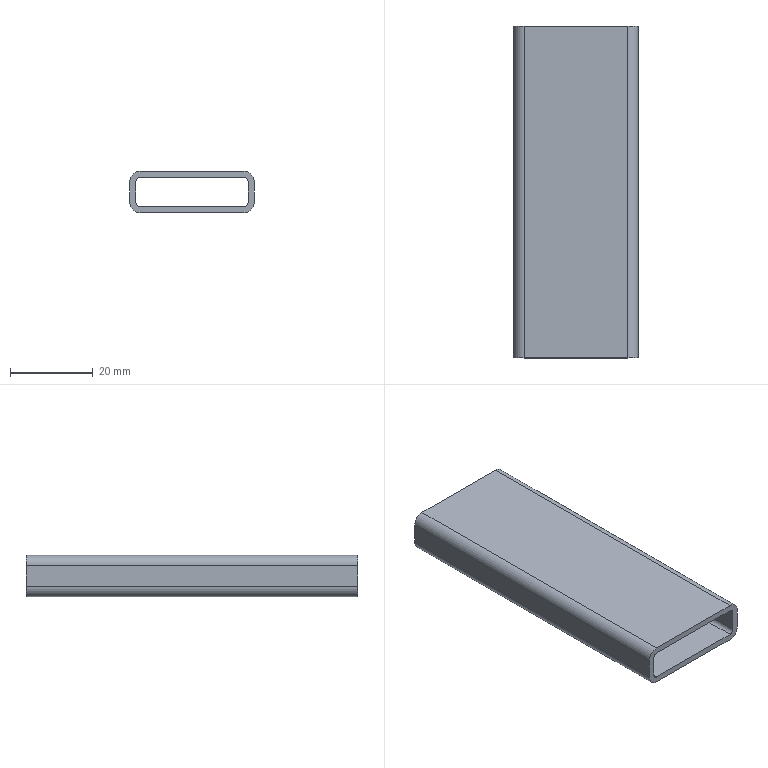Part | STEP file | 7100109 | 1 solid | 18 faces | box 30 x 80 x 10 mm | volume 8519 mm3 | plane 10 | cylinder 8 | commonest cylinder face diameters 2 x4 5 x4
STEP:
#1=CARTESIAN_POINT('',(0.,0.,0.));
#2=DIRECTION('',(0.,0.,1.));
#3=DIRECTION('',(1.,0.,0.));
#4=AXIS2_PLACEMENT_3D('',#1,#2,#3);
#5=CARTESIAN_POINT('',(6.674,80.,-4.725));
#6=VERTEX_POINT('',#5);
#7=CARTESIAN_POINT('',(9.174,80.,-2.225));
#8=VERTEX_POINT('',#7);
#9=CARTESIAN_POINT('',(9.174,80.,-4.725));
#10=DIRECTION('',(0.,1.,0.));
#11=DIRECTION('',(0.,0.,1.));
#12=AXIS2_PLACEMENT_3D('',#9,#10,#11);
#13=CIRCLE('',#12,2.5);
#14=CARTESIAN_POINT('',(9.174,80.,-4.725));
#15=DIRECTION('',(0.,1.,0.));
#16=DIRECTION('',(0.,0.,1.));
#17=AXIS2_PLACEMENT_3D('',#14,#15,#16);
#18=PLANE('',#17);
#19=CARTESIAN_POINT('',(0.,0.));
#20=DIRECTION('',(1.,0.));
#21=AXIS2_PLACEMENT_2D('',#19,#20);
#22=CIRCLE('',#21,2.5);
#23=(GEOMETRIC_REPRESENTATION_CONTEXT(2)PARAMETRIC_REPRESENTATION_CONTEXT()REPRESENTATION_CONTEXT('',''));
#24=DEFINITIONAL_REPRESENTATION('',(#22),#23);
#25=PCURVE('',#18,#24);
#26=CARTESIAN_POINT('',(9.174,80.,-4.725));
#27=DIRECTION('',(0.,-1.,0.));
#28=DIRECTION('',(0.,0.,-1.));
#29=AXIS2_PLACEMENT_3D('',#26,#27,#28);
#30=CYLINDRICAL_SURFACE('',#29,2.5);
#31=CARTESIAN_POINT('',(9.425,0.));
#32=DIRECTION('',(-1.,0.));
#33=VECTOR('',#32,1.);
#34=LINE('',#31,#33);
#35=(GEOMETRIC_REPRESENTATION_CONTEXT(2)PARAMETRIC_REPRESENTATION_CONTEXT()REPRESENTATION_CONTEXT('',''));
#36=DEFINITIONAL_REPRESENTATION('',(#34),#35);
#37=PCURVE('',#30,#36);
#38=SURFACE_CURVE('',#13,(#25,#37),.PCURVE_S1.);
#39=EDGE_CURVE('',#6,#8,#38,.T.);
#40=ORIENTED_EDGE('',*,*,#39,.T.);
#41=CARTESIAN_POINT('',(34.174,80.,-2.225));
#42=VERTEX_POINT('',#41);
#43=CARTESIAN_POINT('',(9.174,80.,-2.225));
#44=DIRECTION('',(1.,0.,0.));
#45=VECTOR('',#44,1.);
#46=LINE('',#43,#45);
#47=CARTESIAN_POINT('',(2.5,0.));
#48=DIRECTION('',(0.,1.));
#49=VECTOR('',#48,1.);
#50=LINE('',#47,#49);
#51=(GEOMETRIC_REPRESENTATION_CONTEXT(2)PARAMETRIC_REPRESENTATION_CONTEXT()REPRESENTATION_CONTEXT('',''));
#52=DEFINITIONAL_REPRESENTATION('',(#50),#51);
#53=PCURVE('',#18,#52);
#54=CARTESIAN_POINT('',(9.174,80.,-2.225));
#55=DIRECTION('',(0.,0.,-1.));
#56=DIRECTION('',(-1.,0.,0.));
#57=AXIS2_PLACEMENT_3D('',#54,#55,#56);
#58=PLANE('',#57);
#59=CARTESIAN_POINT('',(0.,0.));
#60=DIRECTION('',(-1.,0.));
#61=VECTOR('',#60,1.);
#62=LINE('',#59,#61);
#63=(GEOMETRIC_REPRESENTATION_CONTEXT(2)PARAMETRIC_REPRESENTATION_CONTEXT()REPRESENTATION_CONTEXT('',''));
#64=DEFINITIONAL_REPRESENTATION('',(#62),#63);
#65=PCURVE('',#58,#64);
#66=SURFACE_CURVE('',#46,(#53,#65),.PCURVE_S1.);
#67=EDGE_CURVE('',#8,#42,#66,.T.);
#68=ORIENTED_EDGE('',*,*,#67,.T.);
#69=CARTESIAN_POINT('',(36.674,80.,-4.725));
#70=VERTEX_POINT('',#69);
#71=CARTESIAN_POINT('',(34.174,80.,-4.725));
#72=DIRECTION('',(0.,1.,0.));
#73=DIRECTION('',(0.,0.,1.));
#74=AXIS2_PLACEMENT_3D('',#71,#72,#73);
#75=CIRCLE('',#74,2.5);
#76=CARTESIAN_POINT('',(0.,25.));
#77=DIRECTION('',(1.,0.));
#78=AXIS2_PLACEMENT_2D('',#76,#77);
#79=CIRCLE('',#78,2.5);
#80=(GEOMETRIC_REPRESENTATION_CONTEXT(2)PARAMETRIC_REPRESENTATION_CONTEXT()REPRESENTATION_CONTEXT('',''));
#81=DEFINITIONAL_REPRESENTATION('',(#79),#80);
#82=PCURVE('',#18,#81);
#83=CARTESIAN_POINT('',(34.174,80.,-4.725));
#84=DIRECTION('',(0.,-1.,0.));
#85=DIRECTION('',(0.,0.,-1.));
#86=AXIS2_PLACEMENT_3D('',#83,#84,#85);
#87=CYLINDRICAL_SURFACE('',#86,2.5);
#88=CARTESIAN_POINT('',(3.142,0.));
#89=DIRECTION('',(-1.,0.));
#90=VECTOR('',#89,1.);
#91=LINE('',#88,#90);
#92=(GEOMETRIC_REPRESENTATION_CONTEXT(2)PARAMETRIC_REPRESENTATION_CONTEXT()REPRESENTATION_CONTEXT('',''));
#93=DEFINITIONAL_REPRESENTATION('',(#91),#92);
#94=PCURVE('',#87,#93);
#95=SURFACE_CURVE('',#75,(#82,#94),.PCURVE_S1.);
#96=EDGE_CURVE('',#42,#70,#95,.T.);
#97=ORIENTED_EDGE('',*,*,#96,.T.);
#98=CARTESIAN_POINT('',(36.674,80.,-9.725));
#99=VERTEX_POINT('',#98);
#100=CARTESIAN_POINT('',(36.674,80.,-9.725));
#101=DIRECTION('',(0.,0.,-1.));
#102=VECTOR('',#101,1.);
#103=LINE('',#100,#102);
#104=CARTESIAN_POINT('',(-5.,27.5));
#105=DIRECTION('',(-1.,0.));
#106=VECTOR('',#105,1.);
#107=LINE('',#104,#106);
#108=(GEOMETRIC_REPRESENTATION_CONTEXT(2)PARAMETRIC_REPRESENTATION_CONTEXT()REPRESENTATION_CONTEXT('',''));
#109=DEFINITIONAL_REPRESENTATION('',(#107),#108);
#110=PCURVE('',#18,#109);
#111=CARTESIAN_POINT('',(36.674,80.,-9.725));
#112=DIRECTION('',(-1.,0.,0.));
#113=DIRECTION('',(0.,0.,1.));
#114=AXIS2_PLACEMENT_3D('',#111,#112,#113);
#115=PLANE('',#114);
#116=CARTESIAN_POINT('',(0.,0.));
#117=DIRECTION('',(-1.,0.));
#118=VECTOR('',#117,1.);
#119=LINE('',#116,#118);
#120=(GEOMETRIC_REPRESENTATION_CONTEXT(2)PARAMETRIC_REPRESENTATION_CONTEXT()REPRESENTATION_CONTEXT('',''));
#121=DEFINITIONAL_REPRESENTATION('',(#119),#120);
#122=PCURVE('',#115,#121);
#123=SURFACE_CURVE('',#103,(#110,#122),.PCURVE_S1.);
#124=EDGE_CURVE('',#70,#99,#123,.T.);
#125=ORIENTED_EDGE('',*,*,#124,.T.);
#126=CARTESIAN_POINT('',(34.174,80.,-12.225));
#127=VERTEX_POINT('',#126);
#128=CARTESIAN_POINT('',(34.174,80.,-9.725));
#129=DIRECTION('',(0.,1.,0.));
#130=DIRECTION('',(0.,0.,-1.));
#131=AXIS2_PLACEMENT_3D('',#128,#129,#130);
#132=CIRCLE('',#131,2.5);
#133=CARTESIAN_POINT('',(-5.,25.));
#134=DIRECTION('',(-1.,0.));
#135=AXIS2_PLACEMENT_2D('',#133,#134);
#136=CIRCLE('',#135,2.5);
#137=(GEOMETRIC_REPRESENTATION_CONTEXT(2)PARAMETRIC_REPRESENTATION_CONTEXT()REPRESENTATION_CONTEXT('',''));
#138=DEFINITIONAL_REPRESENTATION('',(#136),#137);
#139=PCURVE('',#18,#138);
#140=CARTESIAN_POINT('',(34.174,80.,-9.725));
#141=DIRECTION('',(0.,-1.,0.));
#142=DIRECTION('',(0.,0.,-1.));
#143=AXIS2_PLACEMENT_3D('',#140,#141,#142);
#144=CYLINDRICAL_SURFACE('',#143,2.5);
#145=CARTESIAN_POINT('',(6.283,0.));
#146=DIRECTION('',(-1.,0.));
#147=VECTOR('',#146,1.);
#148=LINE('',#145,#147);
#149=(GEOMETRIC_REPRESENTATION_CONTEXT(2)PARAMETRIC_REPRESENTATION_CONTEXT()REPRESENTATION_CONTEXT('',''));
#150=DEFINITIONAL_REPRESENTATION('',(#148),#149);
#151=PCURVE('',#144,#150);
#152=SURFACE_CURVE('',#132,(#139,#151),.PCURVE_S1.);
#153=EDGE_CURVE('',#99,#127,#152,.T.);
#154=ORIENTED_EDGE('',*,*,#153,.T.);
#155=CARTESIAN_POINT('',(9.174,80.,-12.225));
#156=VERTEX_POINT('',#155);
#157=CARTESIAN_POINT('',(9.174,80.,-12.225));
#158=DIRECTION('',(-1.,0.,0.));
#159=VECTOR('',#158,1.);
#160=LINE('',#157,#159);
#161=CARTESIAN_POINT('',(-7.5,0.));
#162=DIRECTION('',(0.,-1.));
#163=VECTOR('',#162,1.);
#164=LINE('',#161,#163);
#165=(GEOMETRIC_REPRESENTATION_CONTEXT(2)PARAMETRIC_REPRESENTATION_CONTEXT()REPRESENTATION_CONTEXT('',''));
#166=DEFINITIONAL_REPRESENTATION('',(#164),#165);
#167=PCURVE('',#18,#166);
#168=CARTESIAN_POINT('',(9.174,80.,-12.225));
#169=DIRECTION('',(0.,0.,1.));
#170=DIRECTION('',(1.,0.,0.));
#171=AXIS2_PLACEMENT_3D('',#168,#169,#170);
#172=PLANE('',#171);
#173=CARTESIAN_POINT('',(0.,0.));
#174=DIRECTION('',(-1.,0.));
#175=VECTOR('',#174,1.);
#176=LINE('',#173,#175);
#177=(GEOMETRIC_REPRESENTATION_CONTEXT(2)PARAMETRIC_REPRESENTATION_CONTEXT()REPRESENTATION_CONTEXT('',''));
#178=DEFINITIONAL_REPRESENTATION('',(#176),#177);
#179=PCURVE('',#172,#178);
#180=SURFACE_CURVE('',#160,(#167,#179),.PCURVE_S1.);
#181=EDGE_CURVE('',#127,#156,#180,.T.);
#182=ORIENTED_EDGE('',*,*,#181,.T.);
#183=CARTESIAN_POINT('',(6.674,80.,-9.725));
#184=VERTEX_POINT('',#183);
#185=CARTESIAN_POINT('',(9.174,80.,-9.725));
#186=DIRECTION('',(0.,1.,0.));
#187=DIRECTION('',(0.,0.,1.));
#188=AXIS2_PLACEMENT_3D('',#185,#186,#187);
#189=CIRCLE('',#188,2.5);
#190=CARTESIAN_POINT('',(-5.,0.));
#191=DIRECTION('',(1.,0.));
#192=AXIS2_PLACEMENT_2D('',#190,#191);
#193=CIRCLE('',#192,2.5);
#194=(GEOMETRIC_REPRESENTATION_CONTEXT(2)PARAMETRIC_REPRESENTATION_CONTEXT()REPRESENTATION_CONTEXT('',''));
#195=DEFINITIONAL_REPRESENTATION('',(#193),#194);
#196=PCURVE('',#18,#195);
#197=CARTESIAN_POINT('',(9.174,80.,-9.725));
#198=DIRECTION('',(0.,-1.,0.));
#199=DIRECTION('',(0.,0.,-1.));
#200=AXIS2_PLACEMENT_3D('',#197,#198,#199);
#201=CYLINDRICAL_SURFACE('',#200,2.5);
#202=CARTESIAN_POINT('',(9.425,0.));
#203=DIRECTION('',(-1.,0.));
#204=VECTOR('',#203,1.);
#205=LINE('',#202,#204);
#206=(GEOMETRIC_REPRESENTATION_CONTEXT(2)PARAMETRIC_REPRESENTATION_CONTEXT()REPRESENTATION_CONTEXT('',''));
#207=DEFINITIONAL_REPRESENTATION('',(#205),#206);
#208=PCURVE('',#201,#207);
#209=SURFACE_CURVE('',#189,(#196,#208),.PCURVE_S1.);
#210=EDGE_CURVE('',#156,#184,#209,.T.);
#211=ORIENTED_EDGE('',*,*,#210,.T.);
#212=CARTESIAN_POINT('',(6.674,80.,-9.725));
#213=DIRECTION('',(0.,0.,1.));
#214=VECTOR('',#213,1.);
#215=LINE('',#212,#214);
#216=CARTESIAN_POINT('',(-5.,-2.5));
#217=DIRECTION('',(1.,0.));
#218=VECTOR('',#217,1.);
#219=LINE('',#216,#218);
#220=(GEOMETRIC_REPRESENTATION_CONTEXT(2)PARAMETRIC_REPRESENTATION_CONTEXT()REPRESENTATION_CONTEXT('',''));
#221=DEFINITIONAL_REPRESENTATION('',(#219),#220);
#222=PCURVE('',#18,#221);
#223=CARTESIAN_POINT('',(6.674,80.,-9.725));
#224=DIRECTION('',(1.,0.,0.));
#225=DIRECTION('',(0.,0.,-1.));
#226=AXIS2_PLACEMENT_3D('',#223,#224,#225);
#227=PLANE('',#226);
#228=CARTESIAN_POINT('',(0.,0.));
#229=DIRECTION('',(-1.,0.));
#230=VECTOR('',#229,1.);
#231=LINE('',#228,#230);
#232=(GEOMETRIC_REPRESENTATION_CONTEXT(2)PARAMETRIC_REPRESENTATION_CONTEXT()REPRESENTATION_CONTEXT('',''));
#233=DEFINITIONAL_REPRESENTATION('',(#231),#232);
#234=PCURVE('',#227,#233);
#235=SURFACE_CURVE('',#215,(#222,#234),.PCURVE_S1.);
#236=EDGE_CURVE('',#184,#6,#235,.T.);
#237=ORIENTED_EDGE('',*,*,#236,.T.);
#238=EDGE_LOOP('',(#40,#68,#97,#125,#154,#182,#211,#237));
#239=FACE_BOUND('',#238,.T.);
#240=CARTESIAN_POINT('',(8.174,80.,-9.725));
#241=VERTEX_POINT('',#240);
#242=CARTESIAN_POINT('',(8.174,80.,-4.725));
#243=VERTEX_POINT('',#242);
#244=CARTESIAN_POINT('',(8.174,80.,-9.725));
#245=DIRECTION('',(0.,0.,1.));
#246=VECTOR('',#245,1.);
#247=LINE('',#244,#246);
#248=CARTESIAN_POINT('',(-5.,-1.));
#249=DIRECTION('',(1.,0.));
#250=VECTOR('',#249,1.);
#251=LINE('',#248,#250);
#252=(GEOMETRIC_REPRESENTATION_CONTEXT(2)PARAMETRIC_REPRESENTATION_CONTEXT()REPRESENTATION_CONTEXT('',''));
#253=DEFINITIONAL_REPRESENTATION('',(#251),#252);
#254=PCURVE('',#18,#253);
#255=CARTESIAN_POINT('',(8.174,80.,-9.725));
#256=DIRECTION('',(1.,0.,0.));
#257=DIRECTION('',(0.,0.,-1.));
#258=AXIS2_PLACEMENT_3D('',#255,#256,#257);
#259=PLANE('',#258);
#260=CARTESIAN_POINT('',(0.,0.));
#261=DIRECTION('',(-1.,0.));
#262=VECTOR('',#261,1.);
#263=LINE('',#260,#262);
#264=(GEOMETRIC_REPRESENTATION_CONTEXT(2)PARAMETRIC_REPRESENTATION_CONTEXT()REPRESENTATION_CONTEXT('',''));
#265=DEFINITIONAL_REPRESENTATION('',(#263),#264);
#266=PCURVE('',#259,#265);
#267=SURFACE_CURVE('',#247,(#254,#266),.PCURVE_S1.);
#268=EDGE_CURVE('',#241,#243,#267,.T.);
#269=ORIENTED_EDGE('',*,*,#268,.F.);
#270=CARTESIAN_POINT('',(9.174,80.,-10.725));
#271=VERTEX_POINT('',#270);
#272=CARTESIAN_POINT('',(9.174,80.,-9.725));
#273=DIRECTION('',(0.,1.,0.));
#274=DIRECTION('',(0.,0.,1.));
#275=AXIS2_PLACEMENT_3D('',#272,#273,#274);
#276=CIRCLE('',#275,1.);
#277=CARTESIAN_POINT('',(-5.,0.));
#278=DIRECTION('',(1.,0.));
#279=AXIS2_PLACEMENT_2D('',#277,#278);
#280=CIRCLE('',#279,1.);
#281=(GEOMETRIC_REPRESENTATION_CONTEXT(2)PARAMETRIC_REPRESENTATION_CONTEXT()REPRESENTATION_CONTEXT('',''));
#282=DEFINITIONAL_REPRESENTATION('',(#280),#281);
#283=PCURVE('',#18,#282);
#284=CARTESIAN_POINT('',(9.174,80.,-9.725));
#285=DIRECTION('',(0.,-1.,0.));
#286=DIRECTION('',(0.,0.,-1.));
#287=AXIS2_PLACEMENT_3D('',#284,#285,#286);
#288=CYLINDRICAL_SURFACE('',#287,1.);
#289=CARTESIAN_POINT('',(9.425,0.));
#290=DIRECTION('',(-1.,0.));
#291=VECTOR('',#290,1.);
#292=LINE('',#289,#291);
#293=(GEOMETRIC_REPRESENTATION_CONTEXT(2)PARAMETRIC_REPRESENTATION_CONTEXT()REPRESENTATION_CONTEXT('',''));
#294=DEFINITIONAL_REPRESENTATION('',(#292),#293);
#295=PCURVE('',#288,#294);
#296=SURFACE_CURVE('',#276,(#283,#295),.PCURVE_S1.);
#297=EDGE_CURVE('',#271,#241,#296,.T.);
#298=ORIENTED_EDGE('',*,*,#297,.F.);
#299=CARTESIAN_POINT('',(34.174,80.,-10.725));
#300=VERTEX_POINT('',#299);
#301=CARTESIAN_POINT('',(9.174,80.,-10.725));
#302=DIRECTION('',(-1.,0.,0.));
#303=VECTOR('',#302,1.);
#304=LINE('',#301,#303);
#305=CARTESIAN_POINT('',(-6.,0.));
#306=DIRECTION('',(0.,-1.));
#307=VECTOR('',#306,1.);
#308=LINE('',#305,#307);
#309=(GEOMETRIC_REPRESENTATION_CONTEXT(2)PARAMETRIC_REPRESENTATION_CONTEXT()REPRESENTATION_CONTEXT('',''));
#310=DEFINITIONAL_REPRESENTATION('',(#308),#309);
#311=PCURVE('',#18,#310);
#312=CARTESIAN_POINT('',(9.174,80.,-10.725));
#313=DIRECTION('',(0.,0.,1.));
#314=DIRECTION('',(1.,0.,0.));
#315=AXIS2_PLACEMENT_3D('',#312,#313,#314);
#316=PLANE('',#315);
#317=CARTESIAN_POINT('',(0.,0.));
#318=DIRECTION('',(-1.,0.));
#319=VECTOR('',#318,1.);
#320=LINE('',#317,#319);
#321=(GEOMETRIC_REPRESENTATION_CONTEXT(2)PARAMETRIC_REPRESENTATION_CONTEXT()REPRESENTATION_CONTEXT('',''));
#322=DEFINITIONAL_REPRESENTATION('',(#320),#321);
#323=PCURVE('',#316,#322);
#324=SURFACE_CURVE('',#304,(#311,#323),.PCURVE_S1.);
#325=EDGE_CURVE('',#300,#271,#324,.T.);
#326=ORIENTED_EDGE('',*,*,#325,.F.);
#327=CARTESIAN_POINT('',(35.174,80.,-9.725));
#328=VERTEX_POINT('',#327);
#329=CARTESIAN_POINT('',(34.174,80.,-9.725));
#330=DIRECTION('',(0.,1.,0.));
#331=DIRECTION('',(0.,0.,-1.));
#332=AXIS2_PLACEMENT_3D('',#329,#330,#331);
#333=CIRCLE('',#332,1.);
#334=CARTESIAN_POINT('',(-5.,25.));
#335=DIRECTION('',(-1.,0.));
#336=AXIS2_PLACEMENT_2D('',#334,#335);
#337=CIRCLE('',#336,1.);
#338=(GEOMETRIC_REPRESENTATION_CONTEXT(2)PARAMETRIC_REPRESENTATION_CONTEXT()REPRESENTATION_CONTEXT('',''));
#339=DEFINITIONAL_REPRESENTATION('',(#337),#338);
#340=PCURVE('',#18,#339);
#341=CARTESIAN_POINT('',(34.174,80.,-9.725));
#342=DIRECTION('',(0.,-1.,0.));
#343=DIRECTION('',(0.,0.,-1.));
#344=AXIS2_PLACEMENT_3D('',#341,#342,#343);
#345=CYLINDRICAL_SURFACE('',#344,1.);
#346=CARTESIAN_POINT('',(6.283,0.));
#347=DIRECTION('',(-1.,0.));
#348=VECTOR('',#347,1.);
#349=LINE('',#346,#348);
#350=(GEOMETRIC_REPRESENTATION_CONTEXT(2)PARAMETRIC_REPRESENTATION_CONTEXT()REPRESENTATION_CONTEXT('',''));
#351=DEFINITIONAL_REPRESENTATION('',(#349),#350);
#352=PCURVE('',#345,#351);
#353=SURFACE_CURVE('',#333,(#340,#352),.PCURVE_S1.);
#354=EDGE_CURVE('',#328,#300,#353,.T.);
#355=ORIENTED_EDGE('',*,*,#354,.F.);
#356=CARTESIAN_POINT('',(35.174,80.,-4.725));
#357=VERTEX_POINT('',#356);
#358=CARTESIAN_POINT('',(35.174,80.,-9.725));
#359=DIRECTION('',(0.,0.,-1.));
#360=VECTOR('',#359,1.);
#361=LINE('',#358,#360);
#362=CARTESIAN_POINT('',(-5.,26.));
#363=DIRECTION('',(-1.,0.));
#364=VECTOR('',#363,1.);
#365=LINE('',#362,#364);
#366=(GEOMETRIC_REPRESENTATION_CONTEXT(2)PARAMETRIC_REPRESENTATION_CONTEXT()REPRESENTATION_CONTEXT('',''));
#367=DEFINITIONAL_REPRESENTATION('',(#365),#366);
#368=PCURVE('',#18,#367);
#369=CARTESIAN_POINT('',(35.174,80.,-9.725));
#370=DIRECTION('',(-1.,0.,0.));
#371=DIRECTION('',(0.,0.,1.));
#372=AXIS2_PLACEMENT_3D('',#369,#370,#371);
#373=PLANE('',#372);
#374=CARTESIAN_POINT('',(0.,0.));
#375=DIRECTION('',(-1.,0.));
#376=VECTOR('',#375,1.);
#377=LINE('',#374,#376);
#378=(GEOMETRIC_REPRESENTATION_CONTEXT(2)PARAMETRIC_REPRESENTATION_CONTEXT()REPRESENTATION_CONTEXT('',''));
#379=DEFINITIONAL_REPRESENTATION('',(#377),#378);
#380=PCURVE('',#373,#379);
#381=SURFACE_CURVE('',#361,(#368,#380),.PCURVE_S1.);
#382=EDGE_CURVE('',#357,#328,#381,.T.);
#383=ORIENTED_EDGE('',*,*,#382,.F.);
#384=CARTESIAN_POINT('',(34.174,80.,-3.725));
#385=VERTEX_POINT('',#384);
#386=CARTESIAN_POINT('',(34.174,80.,-4.725));
#387=DIRECTION('',(0.,1.,0.));
#388=DIRECTION('',(0.,0.,1.));
#389=AXIS2_PLACEMENT_3D('',#386,#387,#388);
#390=CIRCLE('',#389,1.);
#391=CARTESIAN_POINT('',(0.,25.));
#392=DIRECTION('',(1.,0.));
#393=AXIS2_PLACEMENT_2D('',#391,#392);
#394=CIRCLE('',#393,1.);
#395=(GEOMETRIC_REPRESENTATION_CONTEXT(2)PARAMETRIC_REPRESENTATION_CONTEXT()REPRESENTATION_CONTEXT('',''));
#396=DEFINITIONAL_REPRESENTATION('',(#394),#395);
#397=PCURVE('',#18,#396);
#398=CARTESIAN_POINT('',(34.174,80.,-4.725));
#399=DIRECTION('',(0.,-1.,0.));
#400=DIRECTION('',(0.,0.,-1.));
#401=AXIS2_PLACEMENT_3D('',#398,#399,#400);
#402=CYLINDRICAL_SURFACE('',#401,1.);
#403=CARTESIAN_POINT('',(3.142,0.));
#404=DIRECTION('',(-1.,0.));
#405=VECTOR('',#404,1.);
#406=LINE('',#403,#405);
#407=(GEOMETRIC_REPRESENTATION_CONTEXT(2)PARAMETRIC_REPRESENTATION_CONTEXT()REPRESENTATION_CONTEXT('',''));
#408=DEFINITIONAL_REPRESENTATION('',(#406),#407);
#409=PCURVE('',#402,#408);
#410=SURFACE_CURVE('',#390,(#397,#409),.PCURVE_S1.);
#411=EDGE_CURVE('',#385,#357,#410,.T.);
#412=ORIENTED_EDGE('',*,*,#411,.F.);
#413=CARTESIAN_POINT('',(9.174,80.,-3.725));
#414=VERTEX_POINT('',#413);
#415=CARTESIAN_POINT('',(9.174,80.,-3.725));
#416=DIRECTION('',(1.,0.,0.));
#417=VECTOR('',#416,1.);
#418=LINE('',#415,#417);
#419=CARTESIAN_POINT('',(1.,0.));
#420=DIRECTION('',(0.,1.));
#421=VECTOR('',#420,1.);
#422=LINE('',#419,#421);
#423=(GEOMETRIC_REPRESENTATION_CONTEXT(2)PARAMETRIC_REPRESENTATION_CONTEXT()REPRESENTATION_CONTEXT('',''));
#424=DEFINITIONAL_REPRESENTATION('',(#422),#423);
#425=PCURVE('',#18,#424);
#426=CARTESIAN_POINT('',(9.174,80.,-3.725));
#427=DIRECTION('',(0.,0.,-1.));
#428=DIRECTION('',(-1.,0.,0.));
#429=AXIS2_PLACEMENT_3D('',#426,#427,#428);
#430=PLANE('',#429);
#431=CARTESIAN_POINT('',(0.,0.));
#432=DIRECTION('',(-1.,0.));
#433=VECTOR('',#432,1.);
#434=LINE('',#431,#433);
#435=(GEOMETRIC_REPRESENTATION_CONTEXT(2)PARAMETRIC_REPRESENTATION_CONTEXT()REPRESENTATION_CONTEXT('',''));
#436=DEFINITIONAL_REPRESENTATION('',(#434),#435);
#437=PCURVE('',#430,#436);
#438=SURFACE_CURVE('',#418,(#425,#437),.PCURVE_S1.);
#439=EDGE_CURVE('',#414,#385,#438,.T.);
#440=ORIENTED_EDGE('',*,*,#439,.F.);
#441=CARTESIAN_POINT('',(9.174,80.,-4.725));
#442=DIRECTION('',(0.,1.,0.));
#443=DIRECTION('',(0.,0.,1.));
#444=AXIS2_PLACEMENT_3D('',#441,#442,#443);
#445=CIRCLE('',#444,1.);
#446=CARTESIAN_POINT('',(0.,0.));
#447=DIRECTION('',(1.,0.));
#448=AXIS2_PLACEMENT_2D('',#446,#447);
#449=CIRCLE('',#448,1.);
#450=(GEOMETRIC_REPRESENTATION_CONTEXT(2)PARAMETRIC_REPRESENTATION_CONTEXT()REPRESENTATION_CONTEXT('',''));
#451=DEFINITIONAL_REPRESENTATION('',(#449),#450);
#452=PCURVE('',#18,#451);
#453=CARTESIAN_POINT('',(9.174,80.,-4.725));
#454=DIRECTION('',(0.,-1.,0.));
#455=DIRECTION('',(0.,0.,-1.));
#456=AXIS2_PLACEMENT_3D('',#453,#454,#455);
#457=CYLINDRICAL_SURFACE('',#456,1.);
#458=CARTESIAN_POINT('',(9.425,0.));
#459=DIRECTION('',(-1.,0.));
#460=VECTOR('',#459,1.);
#461=LINE('',#458,#460);
#462=(GEOMETRIC_REPRESENTATION_CONTEXT(2)PARAMETRIC_REPRESENTATION_CONTEXT()REPRESENTATION_CONTEXT('',''));
#463=DEFINITIONAL_REPRESENTATION('',(#461),#462);
#464=PCURVE('',#457,#463);
#465=SURFACE_CURVE('',#445,(#452,#464),.PCURVE_S1.);
#466=EDGE_CURVE('',#243,#414,#465,.T.);
#467=ORIENTED_EDGE('',*,*,#466,.F.);
#468=EDGE_LOOP('',(#269,#298,#326,#355,#383,#412,#440,#467));
#469=FACE_BOUND('',#468,.T.);
#470=ADVANCED_FACE('',(#239,#469),#18,.T.);
#471=CARTESIAN_POINT('',(6.674,0.,-4.725));
#472=VERTEX_POINT('',#471);
#473=CARTESIAN_POINT('',(9.174,0.,-2.225));
#474=VERTEX_POINT('',#473);
#475=CARTESIAN_POINT('',(9.174,0.,-4.725));
#476=DIRECTION('',(0.,1.,0.));
#477=DIRECTION('',(0.,0.,1.));
#478=AXIS2_PLACEMENT_3D('',#475,#476,#477);
#479=CIRCLE('',#478,2.5);
#480=CARTESIAN_POINT('',(9.174,0.,-4.725));
#481=DIRECTION('',(0.,1.,0.));
#482=DIRECTION('',(0.,0.,1.));
#483=AXIS2_PLACEMENT_3D('',#480,#481,#482);
#484=PLANE('',#483);
#485=CARTESIAN_POINT('',(0.,0.));
#486=DIRECTION('',(1.,0.));
#487=AXIS2_PLACEMENT_2D('',#485,#486);
#488=CIRCLE('',#487,2.5);
#489=(GEOMETRIC_REPRESENTATION_CONTEXT(2)PARAMETRIC_REPRESENTATION_CONTEXT()REPRESENTATION_CONTEXT('',''));
#490=DEFINITIONAL_REPRESENTATION('',(#488),#489);
#491=PCURVE('',#484,#490);
#492=CARTESIAN_POINT('',(9.425,80.));
#493=DIRECTION('',(-1.,0.));
#494=VECTOR('',#493,1.);
#495=LINE('',#492,#494);
#496=(GEOMETRIC_REPRESENTATION_CONTEXT(2)PARAMETRIC_REPRESENTATION_CONTEXT()REPRESENTATION_CONTEXT('',''));
#497=DEFINITIONAL_REPRESENTATION('',(#495),#496);
#498=PCURVE('',#30,#497);
#499=SURFACE_CURVE('',#479,(#491,#498),.PCURVE_S1.);
#500=EDGE_CURVE('',#472,#474,#499,.T.);
#501=ORIENTED_EDGE('',*,*,#500,.F.);
#502=CARTESIAN_POINT('',(6.674,0.,-9.725));
#503=VERTEX_POINT('',#502);
#504=CARTESIAN_POINT('',(6.674,0.,-9.725));
#505=DIRECTION('',(0.,0.,1.));
#506=VECTOR('',#505,1.);
#507=LINE('',#504,#506);
#508=CARTESIAN_POINT('',(-5.,-2.5));
#509=DIRECTION('',(1.,0.));
#510=VECTOR('',#509,1.);
#511=LINE('',#508,#510);
#512=(GEOMETRIC_REPRESENTATION_CONTEXT(2)PARAMETRIC_REPRESENTATION_CONTEXT()REPRESENTATION_CONTEXT('',''));
#513=DEFINITIONAL_REPRESENTATION('',(#511),#512);
#514=PCURVE('',#484,#513);
#515=CARTESIAN_POINT('',(0.,-80.));
#516=DIRECTION('',(-1.,0.));
#517=VECTOR('',#516,1.);
#518=LINE('',#515,#517);
#519=(GEOMETRIC_REPRESENTATION_CONTEXT(2)PARAMETRIC_REPRESENTATION_CONTEXT()REPRESENTATION_CONTEXT('',''));
#520=DEFINITIONAL_REPRESENTATION('',(#518),#519);
#521=PCURVE('',#227,#520);
#522=SURFACE_CURVE('',#507,(#514,#521),.PCURVE_S1.);
#523=EDGE_CURVE('',#503,#472,#522,.T.);
#524=ORIENTED_EDGE('',*,*,#523,.F.);
#525=CARTESIAN_POINT('',(9.174,0.,-12.225));
#526=VERTEX_POINT('',#525);
#527=CARTESIAN_POINT('',(9.174,0.,-9.725));
#528=DIRECTION('',(0.,1.,0.));
#529=DIRECTION('',(0.,0.,1.));
#530=AXIS2_PLACEMENT_3D('',#527,#528,#529);
#531=CIRCLE('',#530,2.5);
#532=CARTESIAN_POINT('',(-5.,0.));
#533=DIRECTION('',(1.,0.));
#534=AXIS2_PLACEMENT_2D('',#532,#533);
#535=CIRCLE('',#534,2.5);
#536=(GEOMETRIC_REPRESENTATION_CONTEXT(2)PARAMETRIC_REPRESENTATION_CONTEXT()REPRESENTATION_CONTEXT('',''));
#537=DEFINITIONAL_REPRESENTATION('',(#535),#536);
#538=PCURVE('',#484,#537);
#539=CARTESIAN_POINT('',(9.425,80.));
#540=DIRECTION('',(-1.,0.));
#541=VECTOR('',#540,1.);
#542=LINE('',#539,#541);
#543=(GEOMETRIC_REPRESENTATION_CONTEXT(2)PARAMETRIC_REPRESENTATION_CONTEXT()REPRESENTATION_CONTEXT('',''));
#544=DEFINITIONAL_REPRESENTATION('',(#542),#543);
#545=PCURVE('',#201,#544);
#546=SURFACE_CURVE('',#531,(#538,#545),.PCURVE_S1.);
#547=EDGE_CURVE('',#526,#503,#546,.T.);
#548=ORIENTED_EDGE('',*,*,#547,.F.);
#549=CARTESIAN_POINT('',(34.174,0.,-12.225));
#550=VERTEX_POINT('',#549);
#551=CARTESIAN_POINT('',(9.174,0.,-12.225));
#552=DIRECTION('',(-1.,0.,0.));
#553=VECTOR('',#552,1.);
#554=LINE('',#551,#553);
#555=CARTESIAN_POINT('',(-7.5,0.));
#556=DIRECTION('',(0.,-1.));
#557=VECTOR('',#556,1.);
#558=LINE('',#555,#557);
#559=(GEOMETRIC_REPRESENTATION_CONTEXT(2)PARAMETRIC_REPRESENTATION_CONTEXT()REPRESENTATION_CONTEXT('',''));
#560=DEFINITIONAL_REPRESENTATION('',(#558),#559);
#561=PCURVE('',#484,#560);
#562=CARTESIAN_POINT('',(0.,-80.));
#563=DIRECTION('',(-1.,0.));
#564=VECTOR('',#563,1.);
#565=LINE('',#562,#564);
#566=(GEOMETRIC_REPRESENTATION_CONTEXT(2)PARAMETRIC_REPRESENTATION_CONTEXT()REPRESENTATION_CONTEXT('',''));
#567=DEFINITIONAL_REPRESENTATION('',(#565),#566);
#568=PCURVE('',#172,#567);
#569=SURFACE_CURVE('',#554,(#561,#568),.PCURVE_S1.);
#570=EDGE_CURVE('',#550,#526,#569,.T.);
#571=ORIENTED_EDGE('',*,*,#570,.F.);
#572=CARTESIAN_POINT('',(36.674,0.,-9.725));
#573=VERTEX_POINT('',#572);
#574=CARTESIAN_POINT('',(34.174,0.,-9.725));
#575=DIRECTION('',(0.,1.,0.));
#576=DIRECTION('',(0.,0.,-1.));
#577=AXIS2_PLACEMENT_3D('',#574,#575,#576);
#578=CIRCLE('',#577,2.5);
#579=CARTESIAN_POINT('',(-5.,25.));
#580=DIRECTION('',(-1.,0.));
#581=AXIS2_PLACEMENT_2D('',#579,#580);
#582=CIRCLE('',#581,2.5);
#583=(GEOMETRIC_REPRESENTATION_CONTEXT(2)PARAMETRIC_REPRESENTATION_CONTEXT()REPRESENTATION_CONTEXT('',''));
#584=DEFINITIONAL_REPRESENTATION('',(#582),#583);
#585=PCURVE('',#484,#584);
#586=CARTESIAN_POINT('',(6.283,80.));
#587=DIRECTION('',(-1.,0.));
#588=VECTOR('',#587,1.);
#589=LINE('',#586,#588);
#590=(GEOMETRIC_REPRESENTATION_CONTEXT(2)PARAMETRIC_REPRESENTATION_CONTEXT()REPRESENTATION_CONTEXT('',''));
#591=DEFINITIONAL_REPRESENTATION('',(#589),#590);
#592=PCURVE('',#144,#591);
#593=SURFACE_CURVE('',#578,(#585,#592),.PCURVE_S1.);
#594=EDGE_CURVE('',#573,#550,#593,.T.);
#595=ORIENTED_EDGE('',*,*,#594,.F.);
#596=CARTESIAN_POINT('',(36.674,0.,-4.725));
#597=VERTEX_POINT('',#596);
#598=CARTESIAN_POINT('',(36.674,0.,-9.725));
#599=DIRECTION('',(0.,0.,-1.));
#600=VECTOR('',#599,1.);
#601=LINE('',#598,#600);
#602=CARTESIAN_POINT('',(-5.,27.5));
#603=DIRECTION('',(-1.,0.));
#604=VECTOR('',#603,1.);
#605=LINE('',#602,#604);
#606=(GEOMETRIC_REPRESENTATION_CONTEXT(2)PARAMETRIC_REPRESENTATION_CONTEXT()REPRESENTATION_CONTEXT('',''));
#607=DEFINITIONAL_REPRESENTATION('',(#605),#606);
#608=PCURVE('',#484,#607);
#609=CARTESIAN_POINT('',(0.,-80.));
#610=DIRECTION('',(-1.,0.));
#611=VECTOR('',#610,1.);
#612=LINE('',#609,#611);
#613=(GEOMETRIC_REPRESENTATION_CONTEXT(2)PARAMETRIC_REPRESENTATION_CONTEXT()REPRESENTATION_CONTEXT('',''));
#614=DEFINITIONAL_REPRESENTATION('',(#612),#613);
#615=PCURVE('',#115,#614);
#616=SURFACE_CURVE('',#601,(#608,#615),.PCURVE_S1.);
#617=EDGE_CURVE('',#597,#573,#616,.T.);
#618=ORIENTED_EDGE('',*,*,#617,.F.);
#619=CARTESIAN_POINT('',(34.174,0.,-2.225));
#620=VERTEX_POINT('',#619);
#621=CARTESIAN_POINT('',(34.174,0.,-4.725));
#622=DIRECTION('',(0.,1.,0.));
#623=DIRECTION('',(0.,0.,1.));
#624=AXIS2_PLACEMENT_3D('',#621,#622,#623);
#625=CIRCLE('',#624,2.5);
#626=CARTESIAN_POINT('',(0.,25.));
#627=DIRECTION('',(1.,0.));
#628=AXIS2_PLACEMENT_2D('',#626,#627);
#629=CIRCLE('',#628,2.5);
#630=(GEOMETRIC_REPRESENTATION_CONTEXT(2)PARAMETRIC_REPRESENTATION_CONTEXT()REPRESENTATION_CONTEXT('',''));
#631=DEFINITIONAL_REPRESENTATION('',(#629),#630);
#632=PCURVE('',#484,#631);
#633=CARTESIAN_POINT('',(3.142,80.));
#634=DIRECTION('',(-1.,0.));
#635=VECTOR('',#634,1.);
#636=LINE('',#633,#635);
#637=(GEOMETRIC_REPRESENTATION_CONTEXT(2)PARAMETRIC_REPRESENTATION_CONTEXT()REPRESENTATION_CONTEXT('',''));
#638=DEFINITIONAL_REPRESENTATION('',(#636),#637);
#639=PCURVE('',#87,#638);
#640=SURFACE_CURVE('',#625,(#632,#639),.PCURVE_S1.);
#641=EDGE_CURVE('',#620,#597,#640,.T.);
#642=ORIENTED_EDGE('',*,*,#641,.F.);
#643=CARTESIAN_POINT('',(9.174,0.,-2.225));
#644=DIRECTION('',(1.,0.,0.));
#645=VECTOR('',#644,1.);
#646=LINE('',#643,#645);
#647=CARTESIAN_POINT('',(2.5,0.));
#648=DIRECTION('',(0.,1.));
#649=VECTOR('',#648,1.);
#650=LINE('',#647,#649);
#651=(GEOMETRIC_REPRESENTATION_CONTEXT(2)PARAMETRIC_REPRESENTATION_CONTEXT()REPRESENTATION_CONTEXT('',''));
#652=DEFINITIONAL_REPRESENTATION('',(#650),#651);
#653=PCURVE('',#484,#652);
#654=CARTESIAN_POINT('',(0.,-80.));
#655=DIRECTION('',(-1.,0.));
#656=VECTOR('',#655,1.);
#657=LINE('',#654,#656);
#658=(GEOMETRIC_REPRESENTATION_CONTEXT(2)PARAMETRIC_REPRESENTATION_CONTEXT()REPRESENTATION_CONTEXT('',''));
#659=DEFINITIONAL_REPRESENTATION('',(#657),#658);
#660=PCURVE('',#58,#659);
#661=SURFACE_CURVE('',#646,(#653,#660),.PCURVE_S1.);
#662=EDGE_CURVE('',#474,#620,#661,.T.);
#663=ORIENTED_EDGE('',*,*,#662,.F.);
#664=EDGE_LOOP('',(#501,#524,#548,#571,#595,#618,#642,#663));
#665=FACE_BOUND('',#664,.T.);
#666=CARTESIAN_POINT('',(9.174,0.,-10.725));
#667=VERTEX_POINT('',#666);
#668=CARTESIAN_POINT('',(8.174,0.,-9.725));
#669=VERTEX_POINT('',#668);
#670=CARTESIAN_POINT('',(9.174,0.,-9.725));
#671=DIRECTION('',(0.,1.,0.));
#672=DIRECTION('',(0.,0.,1.));
#673=AXIS2_PLACEMENT_3D('',#670,#671,#672);
#674=CIRCLE('',#673,1.);
#675=CARTESIAN_POINT('',(-5.,0.));
#676=DIRECTION('',(1.,0.));
#677=AXIS2_PLACEMENT_2D('',#675,#676);
#678=CIRCLE('',#677,1.);
#679=(GEOMETRIC_REPRESENTATION_CONTEXT(2)PARAMETRIC_REPRESENTATION_CONTEXT()REPRESENTATION_CONTEXT('',''));
#680=DEFINITIONAL_REPRESENTATION('',(#678),#679);
#681=PCURVE('',#484,#680);
#682=CARTESIAN_POINT('',(9.425,80.));
#683=DIRECTION('',(-1.,0.));
#684=VECTOR('',#683,1.);
#685=LINE('',#682,#684);
#686=(GEOMETRIC_REPRESENTATION_CONTEXT(2)PARAMETRIC_REPRESENTATION_CONTEXT()REPRESENTATION_CONTEXT('',''));
#687=DEFINITIONAL_REPRESENTATION('',(#685),#686);
#688=PCURVE('',#288,#687);
#689=SURFACE_CURVE('',#674,(#681,#688),.PCURVE_S1.);
#690=EDGE_CURVE('',#667,#669,#689,.T.);
#691=ORIENTED_EDGE('',*,*,#690,.T.);
#692=CARTESIAN_POINT('',(8.174,0.,-4.725));
#693=VERTEX_POINT('',#692);
#694=CARTESIAN_POINT('',(8.174,0.,-9.725));
#695=DIRECTION('',(0.,0.,1.));
#696=VECTOR('',#695,1.);
#697=LINE('',#694,#696);
#698=CARTESIAN_POINT('',(-5.,-1.));
#699=DIRECTION('',(1.,0.));
#700=VECTOR('',#699,1.);
#701=LINE('',#698,#700);
#702=(GEOMETRIC_REPRESENTATION_CONTEXT(2)PARAMETRIC_REPRESENTATION_CONTEXT()REPRESENTATION_CONTEXT('',''));
#703=DEFINITIONAL_REPRESENTATION('',(#701),#702);
#704=PCURVE('',#484,#703);
#705=CARTESIAN_POINT('',(0.,-80.));
#706=DIRECTION('',(-1.,0.));
#707=VECTOR('',#706,1.);
#708=LINE('',#705,#707);
#709=(GEOMETRIC_REPRESENTATION_CONTEXT(2)PARAMETRIC_REPRESENTATION_CONTEXT()REPRESENTATION_CONTEXT('',''));
#710=DEFINITIONAL_REPRESENTATION('',(#708),#709);
#711=PCURVE('',#259,#710);
#712=SURFACE_CURVE('',#697,(#704,#711),.PCURVE_S1.);
#713=EDGE_CURVE('',#669,#693,#712,.T.);
#714=ORIENTED_EDGE('',*,*,#713,.T.);
#715=CARTESIAN_POINT('',(9.174,0.,-3.725));
#716=VERTEX_POINT('',#715);
#717=CARTESIAN_POINT('',(9.174,0.,-4.725));
#718=DIRECTION('',(0.,1.,0.));
#719=DIRECTION('',(0.,0.,1.));
#720=AXIS2_PLACEMENT_3D('',#717,#718,#719);
#721=CIRCLE('',#720,1.);
#722=CARTESIAN_POINT('',(0.,0.));
#723=DIRECTION('',(1.,0.));
#724=AXIS2_PLACEMENT_2D('',#722,#723);
#725=CIRCLE('',#724,1.);
#726=(GEOMETRIC_REPRESENTATION_CONTEXT(2)PARAMETRIC_REPRESENTATION_CONTEXT()REPRESENTATION_CONTEXT('',''));
#727=DEFINITIONAL_REPRESENTATION('',(#725),#726);
#728=PCURVE('',#484,#727);
#729=CARTESIAN_POINT('',(9.425,80.));
#730=DIRECTION('',(-1.,0.));
#731=VECTOR('',#730,1.);
#732=LINE('',#729,#731);
#733=(GEOMETRIC_REPRESENTATION_CONTEXT(2)PARAMETRIC_REPRESENTATION_CONTEXT()REPRESENTATION_CONTEXT('',''));
#734=DEFINITIONAL_REPRESENTATION('',(#732),#733);
#735=PCURVE('',#457,#734);
#736=SURFACE_CURVE('',#721,(#728,#735),.PCURVE_S1.);
#737=EDGE_CURVE('',#693,#716,#736,.T.);
#738=ORIENTED_EDGE('',*,*,#737,.T.);
#739=CARTESIAN_POINT('',(34.174,0.,-3.725));
#740=VERTEX_POINT('',#739);
#741=CARTESIAN_POINT('',(9.174,0.,-3.725));
#742=DIRECTION('',(1.,0.,0.));
#743=VECTOR('',#742,1.);
#744=LINE('',#741,#743);
#745=CARTESIAN_POINT('',(1.,0.));
#746=DIRECTION('',(0.,1.));
#747=VECTOR('',#746,1.);
#748=LINE('',#745,#747);
#749=(GEOMETRIC_REPRESENTATION_CONTEXT(2)PARAMETRIC_REPRESENTATION_CONTEXT()REPRESENTATION_CONTEXT('',''));
#750=DEFINITIONAL_REPRESENTATION('',(#748),#749);
#751=PCURVE('',#484,#750);
#752=CARTESIAN_POINT('',(0.,-80.));
#753=DIRECTION('',(-1.,0.));
#754=VECTOR('',#753,1.);
#755=LINE('',#752,#754);
#756=(GEOMETRIC_REPRESENTATION_CONTEXT(2)PARAMETRIC_REPRESENTATION_CONTEXT()REPRESENTATION_CONTEXT('',''));
#757=DEFINITIONAL_REPRESENTATION('',(#755),#756);
#758=PCURVE('',#430,#757);
#759=SURFACE_CURVE('',#744,(#751,#758),.PCURVE_S1.);
#760=EDGE_CURVE('',#716,#740,#759,.T.);
#761=ORIENTED_EDGE('',*,*,#760,.T.);
#762=CARTESIAN_POINT('',(35.174,0.,-4.725));
#763=VERTEX_POINT('',#762);
#764=CARTESIAN_POINT('',(34.174,0.,-4.725));
#765=DIRECTION('',(0.,1.,0.));
#766=DIRECTION('',(0.,0.,1.));
#767=AXIS2_PLACEMENT_3D('',#764,#765,#766);
#768=CIRCLE('',#767,1.);
#769=CARTESIAN_POINT('',(0.,25.));
#770=DIRECTION('',(1.,0.));
#771=AXIS2_PLACEMENT_2D('',#769,#770);
#772=CIRCLE('',#771,1.);
#773=(GEOMETRIC_REPRESENTATION_CONTEXT(2)PARAMETRIC_REPRESENTATION_CONTEXT()REPRESENTATION_CONTEXT('',''));
#774=DEFINITIONAL_REPRESENTATION('',(#772),#773);
#775=PCURVE('',#484,#774);
#776=CARTESIAN_POINT('',(3.142,80.));
#777=DIRECTION('',(-1.,0.));
#778=VECTOR('',#777,1.);
#779=LINE('',#776,#778);
#780=(GEOMETRIC_REPRESENTATION_CONTEXT(2)PARAMETRIC_REPRESENTATION_CONTEXT()REPRESENTATION_CONTEXT('',''));
#781=DEFINITIONAL_REPRESENTATION('',(#779),#780);
#782=PCURVE('',#402,#781);
#783=SURFACE_CURVE('',#768,(#775,#782),.PCURVE_S1.);
#784=EDGE_CURVE('',#740,#763,#783,.T.);
#785=ORIENTED_EDGE('',*,*,#784,.T.);
#786=CARTESIAN_POINT('',(35.174,0.,-9.725));
#787=VERTEX_POINT('',#786);
#788=CARTESIAN_POINT('',(35.174,0.,-9.725));
#789=DIRECTION('',(0.,0.,-1.));
#790=VECTOR('',#789,1.);
#791=LINE('',#788,#790);
#792=CARTESIAN_POINT('',(-5.,26.));
#793=DIRECTION('',(-1.,0.));
#794=VECTOR('',#793,1.);
#795=LINE('',#792,#794);
#796=(GEOMETRIC_REPRESENTATION_CONTEXT(2)PARAMETRIC_REPRESENTATION_CONTEXT()REPRESENTATION_CONTEXT('',''));
#797=DEFINITIONAL_REPRESENTATION('',(#795),#796);
#798=PCURVE('',#484,#797);
#799=CARTESIAN_POINT('',(0.,-80.));
#800=DIRECTION('',(-1.,0.));
#801=VECTOR('',#800,1.);
#802=LINE('',#799,#801);
#803=(GEOMETRIC_REPRESENTATION_CONTEXT(2)PARAMETRIC_REPRESENTATION_CONTEXT()REPRESENTATION_CONTEXT('',''));
#804=DEFINITIONAL_REPRESENTATION('',(#802),#803);
#805=PCURVE('',#373,#804);
#806=SURFACE_CURVE('',#791,(#798,#805),.PCURVE_S1.);
#807=EDGE_CURVE('',#763,#787,#806,.T.);
#808=ORIENTED_EDGE('',*,*,#807,.T.);
#809=CARTESIAN_POINT('',(34.174,0.,-10.725));
#810=VERTEX_POINT('',#809);
#811=CARTESIAN_POINT('',(34.174,0.,-9.725));
#812=DIRECTION('',(0.,1.,0.));
#813=DIRECTION('',(0.,0.,-1.));
#814=AXIS2_PLACEMENT_3D('',#811,#812,#813);
#815=CIRCLE('',#814,1.);
#816=CARTESIAN_POINT('',(-5.,25.));
#817=DIRECTION('',(-1.,0.));
#818=AXIS2_PLACEMENT_2D('',#816,#817);
#819=CIRCLE('',#818,1.);
#820=(GEOMETRIC_REPRESENTATION_CONTEXT(2)PARAMETRIC_REPRESENTATION_CONTEXT()REPRESENTATION_CONTEXT('',''));
#821=DEFINITIONAL_REPRESENTATION('',(#819),#820);
#822=PCURVE('',#484,#821);
#823=CARTESIAN_POINT('',(6.283,80.));
#824=DIRECTION('',(-1.,0.));
#825=VECTOR('',#824,1.);
#826=LINE('',#823,#825);
#827=(GEOMETRIC_REPRESENTATION_CONTEXT(2)PARAMETRIC_REPRESENTATION_CONTEXT()REPRESENTATION_CONTEXT('',''));
#828=DEFINITIONAL_REPRESENTATION('',(#826),#827);
#829=PCURVE('',#345,#828);
#830=SURFACE_CURVE('',#815,(#822,#829),.PCURVE_S1.);
#831=EDGE_CURVE('',#787,#810,#830,.T.);
#832=ORIENTED_EDGE('',*,*,#831,.T.);
#833=CARTESIAN_POINT('',(9.174,0.,-10.725));
#834=DIRECTION('',(-1.,0.,0.));
#835=VECTOR('',#834,1.);
#836=LINE('',#833,#835);
#837=CARTESIAN_POINT('',(-6.,0.));
#838=DIRECTION('',(0.,-1.));
#839=VECTOR('',#838,1.);
#840=LINE('',#837,#839);
#841=(GEOMETRIC_REPRESENTATION_CONTEXT(2)PARAMETRIC_REPRESENTATION_CONTEXT()REPRESENTATION_CONTEXT('',''));
#842=DEFINITIONAL_REPRESENTATION('',(#840),#841);
#843=PCURVE('',#484,#842);
#844=CARTESIAN_POINT('',(0.,-80.));
#845=DIRECTION('',(-1.,0.));
#846=VECTOR('',#845,1.);
#847=LINE('',#844,#846);
#848=(GEOMETRIC_REPRESENTATION_CONTEXT(2)PARAMETRIC_REPRESENTATION_CONTEXT()REPRESENTATION_CONTEXT('',''));
#849=DEFINITIONAL_REPRESENTATION('',(#847),#848);
#850=PCURVE('',#316,#849);
#851=SURFACE_CURVE('',#836,(#843,#850),.PCURVE_S1.);
#852=EDGE_CURVE('',#810,#667,#851,.T.);
#853=ORIENTED_EDGE('',*,*,#852,.T.);
#854=EDGE_LOOP('',(#691,#714,#738,#761,#785,#808,#832,#853));
#855=FACE_BOUND('',#854,.T.);
#856=ADVANCED_FACE('',(#665,#855),#484,.F.);
#857=ORIENTED_EDGE('',*,*,#500,.T.);
#858=CARTESIAN_POINT('',(9.174,80.,-2.225));
#859=DIRECTION('',(0.,-1.,0.));
#860=VECTOR('',#859,1.);
#861=LINE('',#858,#860);
#862=CARTESIAN_POINT('',(3.142,0.));
#863=DIRECTION('',(0.,1.));
#864=VECTOR('',#863,1.);
#865=LINE('',#862,#864);
#866=(GEOMETRIC_REPRESENTATION_CONTEXT(2)PARAMETRIC_REPRESENTATION_CONTEXT()REPRESENTATION_CONTEXT('',''));
#867=DEFINITIONAL_REPRESENTATION('',(#865),#866);
#868=PCURVE('',#30,#867);
#869=CARTESIAN_POINT('',(0.,0.));
#870=DIRECTION('',(0.,-1.));
#871=VECTOR('',#870,1.);
#872=LINE('',#869,#871);
#873=(GEOMETRIC_REPRESENTATION_CONTEXT(2)PARAMETRIC_REPRESENTATION_CONTEXT()REPRESENTATION_CONTEXT('',''));
#874=DEFINITIONAL_REPRESENTATION('',(#872),#873);
#875=PCURVE('',#58,#874);
#876=SURFACE_CURVE('',#861,(#868,#875),.PCURVE_S1.);
#877=EDGE_CURVE('',#8,#474,#876,.T.);
#878=ORIENTED_EDGE('',*,*,#877,.F.);
#879=ORIENTED_EDGE('',*,*,#39,.F.);
#880=CARTESIAN_POINT('',(6.674,80.,-4.725));
#881=DIRECTION('',(0.,-1.,0.));
#882=VECTOR('',#881,1.);
#883=LINE('',#880,#882);
#884=CARTESIAN_POINT('',(4.712,0.));
#885=DIRECTION('',(0.,1.));
#886=VECTOR('',#885,1.);
#887=LINE('',#884,#886);
#888=(GEOMETRIC_REPRESENTATION_CONTEXT(2)PARAMETRIC_REPRESENTATION_CONTEXT()REPRESENTATION_CONTEXT('',''));
#889=DEFINITIONAL_REPRESENTATION('',(#887),#888);
#890=PCURVE('',#30,#889);
#891=CARTESIAN_POINT('',(-5.,0.));
#892=DIRECTION('',(0.,-1.));
#893=VECTOR('',#892,1.);
#894=LINE('',#891,#893);
#895=(GEOMETRIC_REPRESENTATION_CONTEXT(2)PARAMETRIC_REPRESENTATION_CONTEXT()REPRESENTATION_CONTEXT('',''));
#896=DEFINITIONAL_REPRESENTATION('',(#894),#895);
#897=PCURVE('',#227,#896);
#898=SURFACE_CURVE('',#883,(#890,#897),.PCURVE_S1.);
#899=EDGE_CURVE('',#6,#472,#898,.T.);
#900=ORIENTED_EDGE('',*,*,#899,.T.);
#901=EDGE_LOOP('',(#857,#878,#879,#900));
#902=FACE_BOUND('',#901,.T.);
#903=ADVANCED_FACE('',(#902),#30,.T.);
#904=ORIENTED_EDGE('',*,*,#662,.T.);
#905=CARTESIAN_POINT('',(34.174,80.,-2.225));
#906=DIRECTION('',(0.,-1.,0.));
#907=VECTOR('',#906,1.);
#908=LINE('',#905,#907);
#909=CARTESIAN_POINT('',(-25.,0.));
#910=DIRECTION('',(0.,-1.));
#911=VECTOR('',#910,1.);
#912=LINE('',#909,#911);
#913=(GEOMETRIC_REPRESENTATION_CONTEXT(2)PARAMETRIC_REPRESENTATION_CONTEXT()REPRESENTATION_CONTEXT('',''));
#914=DEFINITIONAL_REPRESENTATION('',(#912),#913);
#915=PCURVE('',#58,#914);
#916=CARTESIAN_POINT('',(3.142,0.));
#917=DIRECTION('',(0.,1.));
#918=VECTOR('',#917,1.);
#919=LINE('',#916,#918);
#920=(GEOMETRIC_REPRESENTATION_CONTEXT(2)PARAMETRIC_REPRESENTATION_CONTEXT()REPRESENTATION_CONTEXT('',''));
#921=DEFINITIONAL_REPRESENTATION('',(#919),#920);
#922=PCURVE('',#87,#921);
#923=SURFACE_CURVE('',#908,(#915,#922),.PCURVE_S1.);
#924=EDGE_CURVE('',#42,#620,#923,.T.);
#925=ORIENTED_EDGE('',*,*,#924,.F.);
#926=ORIENTED_EDGE('',*,*,#67,.F.);
#927=ORIENTED_EDGE('',*,*,#877,.T.);
#928=EDGE_LOOP('',(#904,#925,#926,#927));
#929=FACE_BOUND('',#928,.T.);
#930=ADVANCED_FACE('',(#929),#58,.F.);
#931=ORIENTED_EDGE('',*,*,#641,.T.);
#932=CARTESIAN_POINT('',(36.674,80.,-4.725));
#933=DIRECTION('',(0.,-1.,0.));
#934=VECTOR('',#933,1.);
#935=LINE('',#932,#934);
#936=CARTESIAN_POINT('',(1.571,0.));
#937=DIRECTION('',(0.,1.));
#938=VECTOR('',#937,1.);
#939=LINE('',#936,#938);
#940=(GEOMETRIC_REPRESENTATION_CONTEXT(2)PARAMETRIC_REPRESENTATION_CONTEXT()REPRESENTATION_CONTEXT('',''));
#941=DEFINITIONAL_REPRESENTATION('',(#939),#940);
#942=PCURVE('',#87,#941);
#943=CARTESIAN_POINT('',(5.,0.));
#944=DIRECTION('',(0.,-1.));
#945=VECTOR('',#944,1.);
#946=LINE('',#943,#945);
#947=(GEOMETRIC_REPRESENTATION_CONTEXT(2)PARAMETRIC_REPRESENTATION_CONTEXT()REPRESENTATION_CONTEXT('',''));
#948=DEFINITIONAL_REPRESENTATION('',(#946),#947);
#949=PCURVE('',#115,#948);
#950=SURFACE_CURVE('',#935,(#942,#949),.PCURVE_S1.);
#951=EDGE_CURVE('',#70,#597,#950,.T.);
#952=ORIENTED_EDGE('',*,*,#951,.F.);
#953=ORIENTED_EDGE('',*,*,#96,.F.);
#954=ORIENTED_EDGE('',*,*,#924,.T.);
#955=EDGE_LOOP('',(#931,#952,#953,#954));
#956=FACE_BOUND('',#955,.T.);
#957=ADVANCED_FACE('',(#956),#87,.T.);
#958=ORIENTED_EDGE('',*,*,#617,.T.);
#959=CARTESIAN_POINT('',(36.674,80.,-9.725));
#960=DIRECTION('',(0.,-1.,0.));
#961=VECTOR('',#960,1.);
#962=LINE('',#959,#961);
#963=CARTESIAN_POINT('',(0.,0.));
#964=DIRECTION('',(0.,-1.));
#965=VECTOR('',#964,1.);
#966=LINE('',#963,#965);
#967=(GEOMETRIC_REPRESENTATION_CONTEXT(2)PARAMETRIC_REPRESENTATION_CONTEXT()REPRESENTATION_CONTEXT('',''));
#968=DEFINITIONAL_REPRESENTATION('',(#966),#967);
#969=PCURVE('',#115,#968);
#970=CARTESIAN_POINT('',(1.571,0.));
#971=DIRECTION('',(0.,1.));
#972=VECTOR('',#971,1.);
#973=LINE('',#970,#972);
#974=(GEOMETRIC_REPRESENTATION_CONTEXT(2)PARAMETRIC_REPRESENTATION_CONTEXT()REPRESENTATION_CONTEXT('',''));
#975=DEFINITIONAL_REPRESENTATION('',(#973),#974);
#976=PCURVE('',#144,#975);
#977=SURFACE_CURVE('',#962,(#969,#976),.PCURVE_S1.);
#978=EDGE_CURVE('',#99,#573,#977,.T.);
#979=ORIENTED_EDGE('',*,*,#978,.F.);
#980=ORIENTED_EDGE('',*,*,#124,.F.);
#981=ORIENTED_EDGE('',*,*,#951,.T.);
#982=EDGE_LOOP('',(#958,#979,#980,#981));
#983=FACE_BOUND('',#982,.T.);
#984=ADVANCED_FACE('',(#983),#115,.F.);
#985=ORIENTED_EDGE('',*,*,#594,.T.);
#986=CARTESIAN_POINT('',(34.174,80.,-12.225));
#987=DIRECTION('',(0.,-1.,0.));
#988=VECTOR('',#987,1.);
#989=LINE('',#986,#988);
#990=CARTESIAN_POINT('',(0.,0.));
#991=DIRECTION('',(0.,1.));
#992=VECTOR('',#991,1.);
#993=LINE('',#990,#992);
#994=(GEOMETRIC_REPRESENTATION_CONTEXT(2)PARAMETRIC_REPRESENTATION_CONTEXT()REPRESENTATION_CONTEXT('',''));
#995=DEFINITIONAL_REPRESENTATION('',(#993),#994);
#996=PCURVE('',#144,#995);
#997=CARTESIAN_POINT('',(25.,0.));
#998=DIRECTION('',(0.,-1.));
#999=VECTOR('',#998,1.);
#1000=LINE('',#997,#999);
#1001=(GEOMETRIC_REPRESENTATION_CONTEXT(2)PARAMETRIC_REPRESENTATION_CONTEXT()REPRESENTATION_CONTEXT('',''));
#1002=DEFINITIONAL_REPRESENTATION('',(#1000),#1001);
#1003=PCURVE('',#172,#1002);
#1004=SURFACE_CURVE('',#989,(#996,#1003),.PCURVE_S1.);
#1005=EDGE_CURVE('',#127,#550,#1004,.T.);
#1006=ORIENTED_EDGE('',*,*,#1005,.F.);
#1007=ORIENTED_EDGE('',*,*,#153,.F.);
#1008=ORIENTED_EDGE('',*,*,#978,.T.);
#1009=EDGE_LOOP('',(#985,#1006,#1007,#1008));
#1010=FACE_BOUND('',#1009,.T.);
#1011=ADVANCED_FACE('',(#1010),#144,.T.);
#1012=ORIENTED_EDGE('',*,*,#570,.T.);
#1013=CARTESIAN_POINT('',(9.174,80.,-12.225));
#1014=DIRECTION('',(0.,-1.,0.));
#1015=VECTOR('',#1014,1.);
#1016=LINE('',#1013,#1015);
#1017=CARTESIAN_POINT('',(0.,0.));
#1018=DIRECTION('',(0.,-1.));
#1019=VECTOR('',#1018,1.);
#1020=LINE('',#1017,#1019);
#1021=(GEOMETRIC_REPRESENTATION_CONTEXT(2)PARAMETRIC_REPRESENTATION_CONTEXT()REPRESENTATION_CONTEXT('',''));
#1022=DEFINITIONAL_REPRESENTATION('',(#1020),#1021);
#1023=PCURVE('',#172,#1022);
#1024=CARTESIAN_POINT('',(6.283,0.));
#1025=DIRECTION('',(0.,1.));
#1026=VECTOR('',#1025,1.);
#1027=LINE('',#1024,#1026);
#1028=(GEOMETRIC_REPRESENTATION_CONTEXT(2)PARAMETRIC_REPRESENTATION_CONTEXT()REPRESENTATION_CONTEXT('',''));
#1029=DEFINITIONAL_REPRESENTATION('',(#1027),#1028);
#1030=PCURVE('',#201,#1029);
#1031=SURFACE_CURVE('',#1016,(#1023,#1030),.PCURVE_S1.);
#1032=EDGE_CURVE('',#156,#526,#1031,.T.);
#1033=ORIENTED_EDGE('',*,*,#1032,.F.);
#1034=ORIENTED_EDGE('',*,*,#181,.F.);
#1035=ORIENTED_EDGE('',*,*,#1005,.T.);
#1036=EDGE_LOOP('',(#1012,#1033,#1034,#1035));
#1037=FACE_BOUND('',#1036,.T.);
#1038=ADVANCED_FACE('',(#1037),#172,.F.);
#1039=ORIENTED_EDGE('',*,*,#547,.T.);
#1040=CARTESIAN_POINT('',(6.674,80.,-9.725));
#1041=DIRECTION('',(0.,-1.,0.));
#1042=VECTOR('',#1041,1.);
#1043=LINE('',#1040,#1042);
#1044=CARTESIAN_POINT('',(4.712,0.));
#1045=DIRECTION('',(0.,1.));
#1046=VECTOR('',#1045,1.);
#1047=LINE('',#1044,#1046);
#1048=(GEOMETRIC_REPRESENTATION_CONTEXT(2)PARAMETRIC_REPRESENTATION_CONTEXT()REPRESENTATION_CONTEXT('',''));
#1049=DEFINITIONAL_REPRESENTATION('',(#1047),#1048);
#1050=PCURVE('',#201,#1049);
#1051=CARTESIAN_POINT('',(0.,0.));
#1052=DIRECTION('',(0.,-1.));
#1053=VECTOR('',#1052,1.);
#1054=LINE('',#1051,#1053);
#1055=(GEOMETRIC_REPRESENTATION_CONTEXT(2)PARAMETRIC_REPRESENTATION_CONTEXT()REPRESENTATION_CONTEXT('',''));
#1056=DEFINITIONAL_REPRESENTATION('',(#1054),#1055);
#1057=PCURVE('',#227,#1056);
#1058=SURFACE_CURVE('',#1043,(#1050,#1057),.PCURVE_S1.);
#1059=EDGE_CURVE('',#184,#503,#1058,.T.);
#1060=ORIENTED_EDGE('',*,*,#1059,.F.);
#1061=ORIENTED_EDGE('',*,*,#210,.F.);
#1062=ORIENTED_EDGE('',*,*,#1032,.T.);
#1063=EDGE_LOOP('',(#1039,#1060,#1061,#1062));
#1064=FACE_BOUND('',#1063,.T.);
#1065=ADVANCED_FACE('',(#1064),#201,.T.);
#1066=ORIENTED_EDGE('',*,*,#523,.T.);
#1067=ORIENTED_EDGE('',*,*,#899,.F.);
#1068=ORIENTED_EDGE('',*,*,#236,.F.);
#1069=ORIENTED_EDGE('',*,*,#1059,.T.);
#1070=EDGE_LOOP('',(#1066,#1067,#1068,#1069));
#1071=FACE_BOUND('',#1070,.T.);
#1072=ADVANCED_FACE('',(#1071),#227,.F.);
#1073=CARTESIAN_POINT('',(8.174,80.,-9.725));
#1074=DIRECTION('',(0.,-1.,0.));
#1075=VECTOR('',#1074,1.);
#1076=LINE('',#1073,#1075);
#1077=CARTESIAN_POINT('',(4.712,0.));
#1078=DIRECTION('',(0.,1.));
#1079=VECTOR('',#1078,1.);
#1080=LINE('',#1077,#1079);
#1081=(GEOMETRIC_REPRESENTATION_CONTEXT(2)PARAMETRIC_REPRESENTATION_CONTEXT()REPRESENTATION_CONTEXT('',''));
#1082=DEFINITIONAL_REPRESENTATION('',(#1080),#1081);
#1083=PCURVE('',#288,#1082);
#1084=CARTESIAN_POINT('',(0.,0.));
#1085=DIRECTION('',(0.,-1.));
#1086=VECTOR('',#1085,1.);
#1087=LINE('',#1084,#1086);
#1088=(GEOMETRIC_REPRESENTATION_CONTEXT(2)PARAMETRIC_REPRESENTATION_CONTEXT()REPRESENTATION_CONTEXT('',''));
#1089=DEFINITIONAL_REPRESENTATION('',(#1087),#1088);
#1090=PCURVE('',#259,#1089);
#1091=SURFACE_CURVE('',#1076,(#1083,#1090),.PCURVE_S1.);
#1092=EDGE_CURVE('',#241,#669,#1091,.T.);
#1093=ORIENTED_EDGE('',*,*,#1092,.F.);
#1094=ORIENTED_EDGE('',*,*,#297,.F.);
#1095=CARTESIAN_POINT('',(9.174,80.,-10.725));
#1096=DIRECTION('',(0.,-1.,0.));
#1097=VECTOR('',#1096,1.);
#1098=LINE('',#1095,#1097);
#1099=CARTESIAN_POINT('',(6.283,0.));
#1100=DIRECTION('',(0.,1.));
#1101=VECTOR('',#1100,1.);
#1102=LINE('',#1099,#1101);
#1103=(GEOMETRIC_REPRESENTATION_CONTEXT(2)PARAMETRIC_REPRESENTATION_CONTEXT()REPRESENTATION_CONTEXT('',''));
#1104=DEFINITIONAL_REPRESENTATION('',(#1102),#1103);
#1105=PCURVE('',#288,#1104);
#1106=CARTESIAN_POINT('',(0.,0.));
#1107=DIRECTION('',(0.,-1.));
#1108=VECTOR('',#1107,1.);
#1109=LINE('',#1106,#1108);
#1110=(GEOMETRIC_REPRESENTATION_CONTEXT(2)PARAMETRIC_REPRESENTATION_CONTEXT()REPRESENTATION_CONTEXT('',''));
#1111=DEFINITIONAL_REPRESENTATION('',(#1109),#1110);
#1112=PCURVE('',#316,#1111);
#1113=SURFACE_CURVE('',#1098,(#1105,#1112),.PCURVE_S1.);
#1114=EDGE_CURVE('',#271,#667,#1113,.T.);
#1115=ORIENTED_EDGE('',*,*,#1114,.T.);
#1116=ORIENTED_EDGE('',*,*,#690,.T.);
#1117=EDGE_LOOP('',(#1093,#1094,#1115,#1116));
#1118=FACE_BOUND('',#1117,.F.);
#1119=ADVANCED_FACE('',(#1118),#288,.F.);
#1120=ORIENTED_EDGE('',*,*,#713,.F.);
#1121=ORIENTED_EDGE('',*,*,#1092,.F.);
#1122=ORIENTED_EDGE('',*,*,#268,.T.);
#1123=CARTESIAN_POINT('',(8.174,80.,-4.725));
#1124=DIRECTION('',(0.,-1.,0.));
#1125=VECTOR('',#1124,1.);
#1126=LINE('',#1123,#1125);
#1127=CARTESIAN_POINT('',(-5.,0.));
#1128=DIRECTION('',(0.,-1.));
#1129=VECTOR('',#1128,1.);
#1130=LINE('',#1127,#1129);
#1131=(GEOMETRIC_REPRESENTATION_CONTEXT(2)PARAMETRIC_REPRESENTATION_CONTEXT()REPRESENTATION_CONTEXT('',''));
#1132=DEFINITIONAL_REPRESENTATION('',(#1130),#1131);
#1133=PCURVE('',#259,#1132);
#1134=CARTESIAN_POINT('',(4.712,0.));
#1135=DIRECTION('',(0.,1.));
#1136=VECTOR('',#1135,1.);
#1137=LINE('',#1134,#1136);
#1138=(GEOMETRIC_REPRESENTATION_CONTEXT(2)PARAMETRIC_REPRESENTATION_CONTEXT()REPRESENTATION_CONTEXT('',''));
#1139=DEFINITIONAL_REPRESENTATION('',(#1137),#1138);
#1140=PCURVE('',#457,#1139);
#1141=SURFACE_CURVE('',#1126,(#1133,#1140),.PCURVE_S1.);
#1142=EDGE_CURVE('',#243,#693,#1141,.T.);
#1143=ORIENTED_EDGE('',*,*,#1142,.T.);
#1144=EDGE_LOOP('',(#1120,#1121,#1122,#1143));
#1145=FACE_BOUND('',#1144,.T.);
#1146=ADVANCED_FACE('',(#1145),#259,.T.);
#1147=CARTESIAN_POINT('',(9.174,80.,-3.725));
#1148=DIRECTION('',(0.,-1.,0.));
#1149=VECTOR('',#1148,1.);
#1150=LINE('',#1147,#1149);
#1151=CARTESIAN_POINT('',(3.142,0.));
#1152=DIRECTION('',(0.,1.));
#1153=VECTOR('',#1152,1.);
#1154=LINE('',#1151,#1153);
#1155=(GEOMETRIC_REPRESENTATION_CONTEXT(2)PARAMETRIC_REPRESENTATION_CONTEXT()REPRESENTATION_CONTEXT('',''));
#1156=DEFINITIONAL_REPRESENTATION('',(#1154),#1155);
#1157=PCURVE('',#457,#1156);
#1158=CARTESIAN_POINT('',(0.,0.));
#1159=DIRECTION('',(0.,-1.));
#1160=VECTOR('',#1159,1.);
#1161=LINE('',#1158,#1160);
#1162=(GEOMETRIC_REPRESENTATION_CONTEXT(2)PARAMETRIC_REPRESENTATION_CONTEXT()REPRESENTATION_CONTEXT('',''));
#1163=DEFINITIONAL_REPRESENTATION('',(#1161),#1162);
#1164=PCURVE('',#430,#1163);
#1165=SURFACE_CURVE('',#1150,(#1157,#1164),.PCURVE_S1.);
#1166=EDGE_CURVE('',#414,#716,#1165,.T.);
#1167=ORIENTED_EDGE('',*,*,#1166,.F.);
#1168=ORIENTED_EDGE('',*,*,#466,.F.);
#1169=ORIENTED_EDGE('',*,*,#1142,.T.);
#1170=ORIENTED_EDGE('',*,*,#737,.T.);
#1171=EDGE_LOOP('',(#1167,#1168,#1169,#1170));
#1172=FACE_BOUND('',#1171,.F.);
#1173=ADVANCED_FACE('',(#1172),#457,.F.);
#1174=ORIENTED_EDGE('',*,*,#760,.F.);
#1175=ORIENTED_EDGE('',*,*,#1166,.F.);
#1176=ORIENTED_EDGE('',*,*,#439,.T.);
#1177=CARTESIAN_POINT('',(34.174,80.,-3.725));
#1178=DIRECTION('',(0.,-1.,0.));
#1179=VECTOR('',#1178,1.);
#1180=LINE('',#1177,#1179);
#1181=CARTESIAN_POINT('',(-25.,0.));
#1182=DIRECTION('',(0.,-1.));
#1183=VECTOR('',#1182,1.);
#1184=LINE('',#1181,#1183);
#1185=(GEOMETRIC_REPRESENTATION_CONTEXT(2)PARAMETRIC_REPRESENTATION_CONTEXT()REPRESENTATION_CONTEXT('',''));
#1186=DEFINITIONAL_REPRESENTATION('',(#1184),#1185);
#1187=PCURVE('',#430,#1186);
#1188=CARTESIAN_POINT('',(3.142,0.));
#1189=DIRECTION('',(0.,1.));
#1190=VECTOR('',#1189,1.);
#1191=LINE('',#1188,#1190);
#1192=(GEOMETRIC_REPRESENTATION_CONTEXT(2)PARAMETRIC_REPRESENTATION_CONTEXT()REPRESENTATION_CONTEXT('',''));
#1193=DEFINITIONAL_REPRESENTATION('',(#1191),#1192);
#1194=PCURVE('',#402,#1193);
#1195=SURFACE_CURVE('',#1180,(#1187,#1194),.PCURVE_S1.);
#1196=EDGE_CURVE('',#385,#740,#1195,.T.);
#1197=ORIENTED_EDGE('',*,*,#1196,.T.);
#1198=EDGE_LOOP('',(#1174,#1175,#1176,#1197));
#1199=FACE_BOUND('',#1198,.T.);
#1200=ADVANCED_FACE('',(#1199),#430,.T.);
#1201=CARTESIAN_POINT('',(35.174,80.,-4.725));
#1202=DIRECTION('',(0.,-1.,0.));
#1203=VECTOR('',#1202,1.);
#1204=LINE('',#1201,#1203);
#1205=CARTESIAN_POINT('',(1.571,0.));
#1206=DIRECTION('',(0.,1.));
#1207=VECTOR('',#1206,1.);
#1208=LINE('',#1205,#1207);
#1209=(GEOMETRIC_REPRESENTATION_CONTEXT(2)PARAMETRIC_REPRESENTATION_CONTEXT()REPRESENTATION_CONTEXT('',''));
#1210=DEFINITIONAL_REPRESENTATION('',(#1208),#1209);
#1211=PCURVE('',#402,#1210);
#1212=CARTESIAN_POINT('',(5.,0.));
#1213=DIRECTION('',(0.,-1.));
#1214=VECTOR('',#1213,1.);
#1215=LINE('',#1212,#1214);
#1216=(GEOMETRIC_REPRESENTATION_CONTEXT(2)PARAMETRIC_REPRESENTATION_CONTEXT()REPRESENTATION_CONTEXT('',''));
#1217=DEFINITIONAL_REPRESENTATION('',(#1215),#1216);
#1218=PCURVE('',#373,#1217);
#1219=SURFACE_CURVE('',#1204,(#1211,#1218),.PCURVE_S1.);
#1220=EDGE_CURVE('',#357,#763,#1219,.T.);
#1221=ORIENTED_EDGE('',*,*,#1220,.F.);
#1222=ORIENTED_EDGE('',*,*,#411,.F.);
#1223=ORIENTED_EDGE('',*,*,#1196,.T.);
#1224=ORIENTED_EDGE('',*,*,#784,.T.);
#1225=EDGE_LOOP('',(#1221,#1222,#1223,#1224));
#1226=FACE_BOUND('',#1225,.F.);
#1227=ADVANCED_FACE('',(#1226),#402,.F.);
#1228=ORIENTED_EDGE('',*,*,#807,.F.);
#1229=ORIENTED_EDGE('',*,*,#1220,.F.);
#1230=ORIENTED_EDGE('',*,*,#382,.T.);
#1231=CARTESIAN_POINT('',(35.174,80.,-9.725));
#1232=DIRECTION('',(0.,-1.,0.));
#1233=VECTOR('',#1232,1.);
#1234=LINE('',#1231,#1233);
#1235=CARTESIAN_POINT('',(0.,0.));
#1236=DIRECTION('',(0.,-1.));
#1237=VECTOR('',#1236,1.);
#1238=LINE('',#1235,#1237);
#1239=(GEOMETRIC_REPRESENTATION_CONTEXT(2)PARAMETRIC_REPRESENTATION_CONTEXT()REPRESENTATION_CONTEXT('',''));
#1240=DEFINITIONAL_REPRESENTATION('',(#1238),#1239);
#1241=PCURVE('',#373,#1240);
#1242=CARTESIAN_POINT('',(1.571,0.));
#1243=DIRECTION('',(0.,1.));
#1244=VECTOR('',#1243,1.);
#1245=LINE('',#1242,#1244);
#1246=(GEOMETRIC_REPRESENTATION_CONTEXT(2)PARAMETRIC_REPRESENTATION_CONTEXT()REPRESENTATION_CONTEXT('',''));
#1247=DEFINITIONAL_REPRESENTATION('',(#1245),#1246);
#1248=PCURVE('',#345,#1247);
#1249=SURFACE_CURVE('',#1234,(#1241,#1248),.PCURVE_S1.);
#1250=EDGE_CURVE('',#328,#787,#1249,.T.);
#1251=ORIENTED_EDGE('',*,*,#1250,.T.);
#1252=EDGE_LOOP('',(#1228,#1229,#1230,#1251));
#1253=FACE_BOUND('',#1252,.T.);
#1254=ADVANCED_FACE('',(#1253),#373,.T.);
#1255=CARTESIAN_POINT('',(34.174,80.,-10.725));
#1256=DIRECTION('',(0.,-1.,0.));
#1257=VECTOR('',#1256,1.);
#1258=LINE('',#1255,#1257);
#1259=CARTESIAN_POINT('',(0.,0.));
#1260=DIRECTION('',(0.,1.));
#1261=VECTOR('',#1260,1.);
#1262=LINE('',#1259,#1261);
#1263=(GEOMETRIC_REPRESENTATION_CONTEXT(2)PARAMETRIC_REPRESENTATION_CONTEXT()REPRESENTATION_CONTEXT('',''));
#1264=DEFINITIONAL_REPRESENTATION('',(#1262),#1263);
#1265=PCURVE('',#345,#1264);
#1266=CARTESIAN_POINT('',(25.,0.));
#1267=DIRECTION('',(0.,-1.));
#1268=VECTOR('',#1267,1.);
#1269=LINE('',#1266,#1268);
#1270=(GEOMETRIC_REPRESENTATION_CONTEXT(2)PARAMETRIC_REPRESENTATION_CONTEXT()REPRESENTATION_CONTEXT('',''));
#1271=DEFINITIONAL_REPRESENTATION('',(#1269),#1270);
#1272=PCURVE('',#316,#1271);
#1273=SURFACE_CURVE('',#1258,(#1265,#1272),.PCURVE_S1.);
#1274=EDGE_CURVE('',#300,#810,#1273,.T.);
#1275=ORIENTED_EDGE('',*,*,#1274,.F.);
#1276=ORIENTED_EDGE('',*,*,#354,.F.);
#1277=ORIENTED_EDGE('',*,*,#1250,.T.);
#1278=ORIENTED_EDGE('',*,*,#831,.T.);
#1279=EDGE_LOOP('',(#1275,#1276,#1277,#1278));
#1280=FACE_BOUND('',#1279,.F.);
#1281=ADVANCED_FACE('',(#1280),#345,.F.);
#1282=ORIENTED_EDGE('',*,*,#852,.F.);
#1283=ORIENTED_EDGE('',*,*,#1274,.F.);
#1284=ORIENTED_EDGE('',*,*,#325,.T.);
#1285=ORIENTED_EDGE('',*,*,#1114,.T.);
#1286=EDGE_LOOP('',(#1282,#1283,#1284,#1285));
#1287=FACE_BOUND('',#1286,.T.);
#1288=ADVANCED_FACE('',(#1287),#316,.T.);
#1289=CLOSED_SHELL('',(#470,#856,#903,#930,#957,#984,#1011,#1038,#1065,#1072,#1119,#1146,#1173,#1200,#1227,#1254,#1281,#1288));
#1290=MANIFOLD_SOLID_BREP('',#1289);
#1291=(LENGTH_UNIT()NAMED_UNIT(*)SI_UNIT(.MILLI.,.METRE.));
#1292=UNCERTAINTY_MEASURE_WITH_UNIT(LENGTH_MEASURE(0.0000001),#1291,'','');
#1293=(NAMED_UNIT(*)PLANE_ANGLE_UNIT()SI_UNIT($,.RADIAN.));
#1294=(NAMED_UNIT(*)SI_UNIT($,.STERADIAN.)SOLID_ANGLE_UNIT());
#1295=(GEOMETRIC_REPRESENTATION_CONTEXT(3)GLOBAL_UNCERTAINTY_ASSIGNED_CONTEXT((#1292))GLOBAL_UNIT_ASSIGNED_CONTEXT((#1291,#1293,#1294))REPRESENTATION_CONTEXT('',''));
#1296=ADVANCED_BREP_SHAPE_REPRESENTATION('',(#4,#1290),#1295);